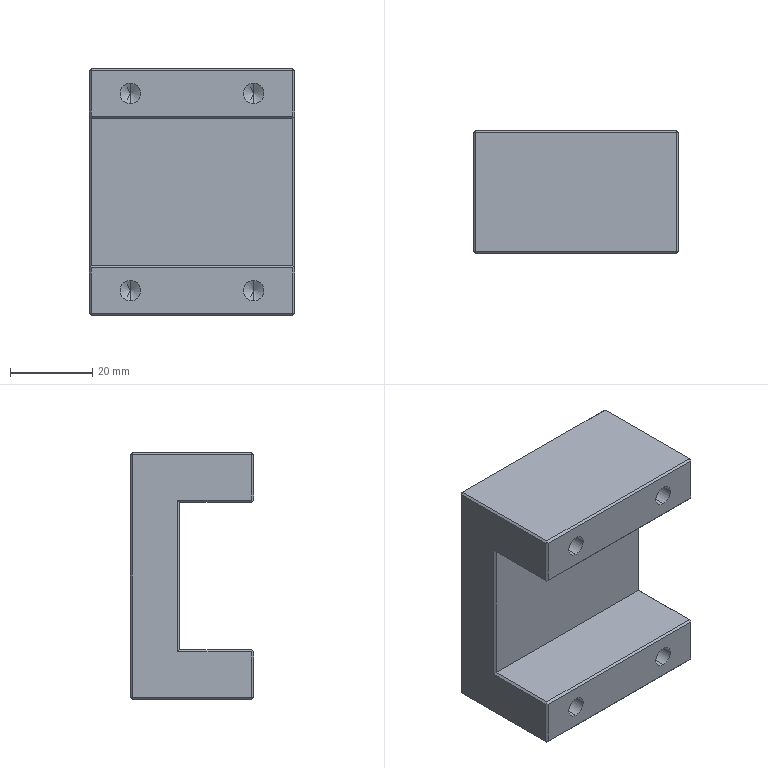Part | SolidWorks | features Chamfer 2, Extrusion 1, HoleWzd 1, ICE 1 | 1 solid | 56 faces | box 50 x 30 x 60 mm | volume 56292 mm3 | plane 40 | cylinder 8 | cone 8 | commonest cylinder face diameters 5 x8
STEP:
#1=CARTESIAN_POINT('',(-15.,15.,-21.5));
#2=VERTEX_POINT('',#1);
#3=CARTESIAN_POINT('',(-15.,15.,-26.5));
#4=VERTEX_POINT('',#3);
#5=CARTESIAN_POINT('',(-15.,15.,-24.));
#6=DIRECTION('',(0.,-1.,0.));
#7=DIRECTION('',(0.,0.,-1.));
#8=AXIS2_PLACEMENT_3D('',#5,#6,#7);
#9=CIRCLE('',#8,2.5);
#10=EDGE_CURVE('',#2,#4,#9,.T.);
#11=ORIENTED_EDGE('',*,*,#10,.F.);
#12=CARTESIAN_POINT('',(-15.,0.,-21.5));
#13=VERTEX_POINT('',#12);
#14=CARTESIAN_POINT('',(-15.,0.,-21.5));
#15=DIRECTION('',(0.,-1.,0.));
#16=VECTOR('',#15,1000.);
#17=LINE('',#14,#16);
#18=EDGE_CURVE('',#2,#13,#17,.T.);
#19=ORIENTED_EDGE('',*,*,#18,.T.);
#20=CARTESIAN_POINT('',(-15.,0.,-26.5));
#21=VERTEX_POINT('',#20);
#22=CARTESIAN_POINT('',(-15.,0.,-24.));
#23=DIRECTION('',(0.,-1.,0.));
#24=DIRECTION('',(0.,0.,-1.));
#25=AXIS2_PLACEMENT_3D('',#22,#23,#24);
#26=CIRCLE('',#25,2.5);
#27=EDGE_CURVE('',#13,#21,#26,.T.);
#28=ORIENTED_EDGE('',*,*,#27,.T.);
#29=CARTESIAN_POINT('',(-15.,0.,-26.5));
#30=DIRECTION('',(0.,-1.,0.));
#31=VECTOR('',#30,1000.);
#32=LINE('',#29,#31);
#33=EDGE_CURVE('',#4,#21,#32,.T.);
#34=ORIENTED_EDGE('',*,*,#33,.F.);
#35=EDGE_LOOP('',(#11,#19,#28,#34));
#36=FACE_OUTER_BOUND('',#35,.T.);
#37=CARTESIAN_POINT('',(-15.,0.,-24.));
#38=DIRECTION('',(0.,-1.,0.));
#39=DIRECTION('',(0.,0.,-1.));
#40=AXIS2_PLACEMENT_3D('',#37,#38,#39);
#41=CYLINDRICAL_SURFACE('',#40,2.5);
#42=ADVANCED_FACE('',(#36),#41,.F.);
#43=CARTESIAN_POINT('',(-15.,16.502,-24.));
#44=VERTEX_POINT('',#43);
#45=CARTESIAN_POINT('',(-15.,15.,-26.5));
#46=DIRECTION('',(0.,-0.515,-0.8572));
#47=VECTOR('',#46,1000.);
#48=LINE('',#45,#47);
#49=EDGE_CURVE('',#44,#4,#48,.T.);
#50=ORIENTED_EDGE('',*,*,#49,.F.);
#51=CARTESIAN_POINT('',(-15.,15.,-21.5));
#52=DIRECTION('',(0.,-0.515,0.8572));
#53=VECTOR('',#52,1000.);
#54=LINE('',#51,#53);
#55=EDGE_CURVE('',#44,#2,#54,.T.);
#56=ORIENTED_EDGE('',*,*,#55,.T.);
#57=ORIENTED_EDGE('',*,*,#10,.T.);
#58=EDGE_LOOP('',(#50,#56,#57));
#59=FACE_OUTER_BOUND('',#58,.T.);
#60=CARTESIAN_POINT('',(-15.,15.,-24.));
#61=DIRECTION('',(0.,-1.,0.));
#62=DIRECTION('',(0.,0.,-1.));
#63=AXIS2_PLACEMENT_3D('',#60,#61,#62);
#64=CONICAL_SURFACE('',#63,2.5,1.03);
#65=ADVANCED_FACE('',(#59),#64,.F.);
#66=CARTESIAN_POINT('',(15.,15.,-21.5));
#67=VERTEX_POINT('',#66);
#68=CARTESIAN_POINT('',(15.,15.,-26.5));
#69=VERTEX_POINT('',#68);
#70=CARTESIAN_POINT('',(15.,15.,-24.));
#71=DIRECTION('',(0.,-1.,0.));
#72=DIRECTION('',(0.,0.,-1.));
#73=AXIS2_PLACEMENT_3D('',#70,#71,#72);
#74=CIRCLE('',#73,2.5);
#75=EDGE_CURVE('',#67,#69,#74,.T.);
#76=ORIENTED_EDGE('',*,*,#75,.F.);
#77=CARTESIAN_POINT('',(15.,0.,-21.5));
#78=VERTEX_POINT('',#77);
#79=CARTESIAN_POINT('',(15.,0.,-21.5));
#80=DIRECTION('',(0.,-1.,0.));
#81=VECTOR('',#80,1000.);
#82=LINE('',#79,#81);
#83=EDGE_CURVE('',#67,#78,#82,.T.);
#84=ORIENTED_EDGE('',*,*,#83,.T.);
#85=CARTESIAN_POINT('',(15.,0.,-26.5));
#86=VERTEX_POINT('',#85);
#87=CARTESIAN_POINT('',(15.,0.,-24.));
#88=DIRECTION('',(0.,-1.,0.));
#89=DIRECTION('',(0.,0.,-1.));
#90=AXIS2_PLACEMENT_3D('',#87,#88,#89);
#91=CIRCLE('',#90,2.5);
#92=EDGE_CURVE('',#78,#86,#91,.T.);
#93=ORIENTED_EDGE('',*,*,#92,.T.);
#94=CARTESIAN_POINT('',(15.,0.,-26.5));
#95=DIRECTION('',(0.,-1.,0.));
#96=VECTOR('',#95,1000.);
#97=LINE('',#94,#96);
#98=EDGE_CURVE('',#69,#86,#97,.T.);
#99=ORIENTED_EDGE('',*,*,#98,.F.);
#100=EDGE_LOOP('',(#76,#84,#93,#99));
#101=FACE_OUTER_BOUND('',#100,.T.);
#102=CARTESIAN_POINT('',(15.,0.,-24.));
#103=DIRECTION('',(0.,-1.,0.));
#104=DIRECTION('',(0.,0.,-1.));
#105=AXIS2_PLACEMENT_3D('',#102,#103,#104);
#106=CYLINDRICAL_SURFACE('',#105,2.5);
#107=ADVANCED_FACE('',(#101),#106,.F.);
#108=CARTESIAN_POINT('',(15.,16.502,-24.));
#109=VERTEX_POINT('',#108);
#110=CARTESIAN_POINT('',(15.,15.,-26.5));
#111=DIRECTION('',(0.,-0.515,-0.8572));
#112=VECTOR('',#111,1000.);
#113=LINE('',#110,#112);
#114=EDGE_CURVE('',#109,#69,#113,.T.);
#115=ORIENTED_EDGE('',*,*,#114,.F.);
#116=CARTESIAN_POINT('',(15.,15.,-21.5));
#117=DIRECTION('',(0.,-0.515,0.8572));
#118=VECTOR('',#117,1000.);
#119=LINE('',#116,#118);
#120=EDGE_CURVE('',#109,#67,#119,.T.);
#121=ORIENTED_EDGE('',*,*,#120,.T.);
#122=ORIENTED_EDGE('',*,*,#75,.T.);
#123=EDGE_LOOP('',(#115,#121,#122));
#124=FACE_OUTER_BOUND('',#123,.T.);
#125=CARTESIAN_POINT('',(15.,15.,-24.));
#126=DIRECTION('',(0.,-1.,0.));
#127=DIRECTION('',(0.,0.,-1.));
#128=AXIS2_PLACEMENT_3D('',#125,#126,#127);
#129=CONICAL_SURFACE('',#128,2.5,1.03);
#130=ADVANCED_FACE('',(#124),#129,.F.);
#131=CARTESIAN_POINT('',(-15.,15.,26.5));
#132=VERTEX_POINT('',#131);
#133=CARTESIAN_POINT('',(-15.,15.,21.5));
#134=VERTEX_POINT('',#133);
#135=CARTESIAN_POINT('',(-15.,15.,24.));
#136=DIRECTION('',(0.,-1.,0.));
#137=DIRECTION('',(0.,0.,-1.));
#138=AXIS2_PLACEMENT_3D('',#135,#136,#137);
#139=CIRCLE('',#138,2.5);
#140=EDGE_CURVE('',#132,#134,#139,.T.);
#141=ORIENTED_EDGE('',*,*,#140,.F.);
#142=CARTESIAN_POINT('',(-15.,0.,26.5));
#143=VERTEX_POINT('',#142);
#144=CARTESIAN_POINT('',(-15.,0.,26.5));
#145=DIRECTION('',(0.,-1.,0.));
#146=VECTOR('',#145,1000.);
#147=LINE('',#144,#146);
#148=EDGE_CURVE('',#132,#143,#147,.T.);
#149=ORIENTED_EDGE('',*,*,#148,.T.);
#150=CARTESIAN_POINT('',(-15.,0.,21.5));
#151=VERTEX_POINT('',#150);
#152=CARTESIAN_POINT('',(-15.,0.,24.));
#153=DIRECTION('',(0.,-1.,0.));
#154=DIRECTION('',(0.,0.,-1.));
#155=AXIS2_PLACEMENT_3D('',#152,#153,#154);
#156=CIRCLE('',#155,2.5);
#157=EDGE_CURVE('',#143,#151,#156,.T.);
#158=ORIENTED_EDGE('',*,*,#157,.T.);
#159=CARTESIAN_POINT('',(-15.,0.,21.5));
#160=DIRECTION('',(0.,-1.,0.));
#161=VECTOR('',#160,1000.);
#162=LINE('',#159,#161);
#163=EDGE_CURVE('',#134,#151,#162,.T.);
#164=ORIENTED_EDGE('',*,*,#163,.F.);
#165=EDGE_LOOP('',(#141,#149,#158,#164));
#166=FACE_OUTER_BOUND('',#165,.T.);
#167=CARTESIAN_POINT('',(-15.,0.,24.));
#168=DIRECTION('',(0.,-1.,0.));
#169=DIRECTION('',(0.,0.,-1.));
#170=AXIS2_PLACEMENT_3D('',#167,#168,#169);
#171=CYLINDRICAL_SURFACE('',#170,2.5);
#172=ADVANCED_FACE('',(#166),#171,.F.);
#173=CARTESIAN_POINT('',(-15.,16.502,24.));
#174=VERTEX_POINT('',#173);
#175=CARTESIAN_POINT('',(-15.,15.,21.5));
#176=DIRECTION('',(0.,-0.515,-0.8572));
#177=VECTOR('',#176,1000.);
#178=LINE('',#175,#177);
#179=EDGE_CURVE('',#174,#134,#178,.T.);
#180=ORIENTED_EDGE('',*,*,#179,.F.);
#181=CARTESIAN_POINT('',(-15.,15.,26.5));
#182=DIRECTION('',(0.,-0.515,0.8572));
#183=VECTOR('',#182,1000.);
#184=LINE('',#181,#183);
#185=EDGE_CURVE('',#174,#132,#184,.T.);
#186=ORIENTED_EDGE('',*,*,#185,.T.);
#187=ORIENTED_EDGE('',*,*,#140,.T.);
#188=EDGE_LOOP('',(#180,#186,#187));
#189=FACE_OUTER_BOUND('',#188,.T.);
#190=CARTESIAN_POINT('',(-15.,15.,24.));
#191=DIRECTION('',(0.,-1.,0.));
#192=DIRECTION('',(0.,0.,-1.));
#193=AXIS2_PLACEMENT_3D('',#190,#191,#192);
#194=CONICAL_SURFACE('',#193,2.5,1.03);
#195=ADVANCED_FACE('',(#189),#194,.F.);
#196=CARTESIAN_POINT('',(15.,15.,26.5));
#197=VERTEX_POINT('',#196);
#198=CARTESIAN_POINT('',(15.,15.,21.5));
#199=VERTEX_POINT('',#198);
#200=CARTESIAN_POINT('',(15.,15.,24.));
#201=DIRECTION('',(0.,-1.,0.));
#202=DIRECTION('',(0.,0.,-1.));
#203=AXIS2_PLACEMENT_3D('',#200,#201,#202);
#204=CIRCLE('',#203,2.5);
#205=EDGE_CURVE('',#197,#199,#204,.T.);
#206=ORIENTED_EDGE('',*,*,#205,.F.);
#207=CARTESIAN_POINT('',(15.,0.,26.5));
#208=VERTEX_POINT('',#207);
#209=CARTESIAN_POINT('',(15.,0.,26.5));
#210=DIRECTION('',(0.,-1.,0.));
#211=VECTOR('',#210,1000.);
#212=LINE('',#209,#211);
#213=EDGE_CURVE('',#197,#208,#212,.T.);
#214=ORIENTED_EDGE('',*,*,#213,.T.);
#215=CARTESIAN_POINT('',(15.,0.,21.5));
#216=VERTEX_POINT('',#215);
#217=CARTESIAN_POINT('',(15.,0.,24.));
#218=DIRECTION('',(0.,-1.,0.));
#219=DIRECTION('',(0.,0.,-1.));
#220=AXIS2_PLACEMENT_3D('',#217,#218,#219);
#221=CIRCLE('',#220,2.5);
#222=EDGE_CURVE('',#208,#216,#221,.T.);
#223=ORIENTED_EDGE('',*,*,#222,.T.);
#224=CARTESIAN_POINT('',(15.,0.,21.5));
#225=DIRECTION('',(0.,-1.,0.));
#226=VECTOR('',#225,1000.);
#227=LINE('',#224,#226);
#228=EDGE_CURVE('',#199,#216,#227,.T.);
#229=ORIENTED_EDGE('',*,*,#228,.F.);
#230=EDGE_LOOP('',(#206,#214,#223,#229));
#231=FACE_OUTER_BOUND('',#230,.T.);
#232=CARTESIAN_POINT('',(15.,0.,24.));
#233=DIRECTION('',(0.,-1.,0.));
#234=DIRECTION('',(0.,0.,-1.));
#235=AXIS2_PLACEMENT_3D('',#232,#233,#234);
#236=CYLINDRICAL_SURFACE('',#235,2.5);
#237=ADVANCED_FACE('',(#231),#236,.F.);
#238=CARTESIAN_POINT('',(15.,16.502,24.));
#239=VERTEX_POINT('',#238);
#240=CARTESIAN_POINT('',(15.,15.,21.5));
#241=DIRECTION('',(0.,-0.515,-0.8572));
#242=VECTOR('',#241,1000.);
#243=LINE('',#240,#242);
#244=EDGE_CURVE('',#239,#199,#243,.T.);
#245=ORIENTED_EDGE('',*,*,#244,.F.);
#246=CARTESIAN_POINT('',(15.,15.,26.5));
#247=DIRECTION('',(0.,-0.515,0.8572));
#248=VECTOR('',#247,1000.);
#249=LINE('',#246,#248);
#250=EDGE_CURVE('',#239,#197,#249,.T.);
#251=ORIENTED_EDGE('',*,*,#250,.T.);
#252=ORIENTED_EDGE('',*,*,#205,.T.);
#253=EDGE_LOOP('',(#245,#251,#252));
#254=FACE_OUTER_BOUND('',#253,.T.);
#255=CARTESIAN_POINT('',(15.,15.,24.));
#256=DIRECTION('',(0.,-1.,0.));
#257=DIRECTION('',(0.,0.,-1.));
#258=AXIS2_PLACEMENT_3D('',#255,#256,#257);
#259=CONICAL_SURFACE('',#258,2.5,1.03);
#260=ADVANCED_FACE('',(#254),#259,.F.);
#261=CARTESIAN_POINT('',(-15.,0.,-24.));
#262=DIRECTION('',(0.,-1.,0.));
#263=DIRECTION('',(0.,0.,-1.));
#264=AXIS2_PLACEMENT_3D('',#261,#262,#263);
#265=CIRCLE('',#264,2.5);
#266=EDGE_CURVE('',#21,#13,#265,.T.);
#267=ORIENTED_EDGE('',*,*,#266,.F.);
#268=ORIENTED_EDGE('',*,*,#27,.F.);
#269=EDGE_LOOP('',(#267,#268));
#270=FACE_BOUND('',#269,.T.);
#271=CARTESIAN_POINT('',(15.,0.,-24.));
#272=DIRECTION('',(0.,-1.,0.));
#273=DIRECTION('',(0.,0.,-1.));
#274=AXIS2_PLACEMENT_3D('',#271,#272,#273);
#275=CIRCLE('',#274,2.5);
#276=EDGE_CURVE('',#86,#78,#275,.T.);
#277=ORIENTED_EDGE('',*,*,#276,.F.);
#278=ORIENTED_EDGE('',*,*,#92,.F.);
#279=EDGE_LOOP('',(#277,#278));
#280=FACE_BOUND('',#279,.T.);
#281=CARTESIAN_POINT('',(24.5,0.,-29.5));
#282=VERTEX_POINT('',#281);
#283=CARTESIAN_POINT('',(24.5,0.,-18.5));
#284=VERTEX_POINT('',#283);
#285=CARTESIAN_POINT('',(24.5,0.,30.));
#286=DIRECTION('',(0.,0.,1.));
#287=VECTOR('',#286,1000.);
#288=LINE('',#285,#287);
#289=EDGE_CURVE('',#282,#284,#288,.T.);
#290=ORIENTED_EDGE('',*,*,#289,.T.);
#291=CARTESIAN_POINT('',(-24.5,0.,-18.5));
#292=VERTEX_POINT('',#291);
#293=CARTESIAN_POINT('',(-24.5,0.,-18.5));
#294=DIRECTION('',(-1.,0.,0.));
#295=VECTOR('',#294,1000.);
#296=LINE('',#293,#295);
#297=EDGE_CURVE('',#284,#292,#296,.T.);
#298=ORIENTED_EDGE('',*,*,#297,.T.);
#299=CARTESIAN_POINT('',(-24.5,0.,-29.5));
#300=VERTEX_POINT('',#299);
#301=CARTESIAN_POINT('',(-24.5,0.,-30.));
#302=DIRECTION('',(0.,0.,-1.));
#303=VECTOR('',#302,1000.);
#304=LINE('',#301,#303);
#305=EDGE_CURVE('',#292,#300,#304,.T.);
#306=ORIENTED_EDGE('',*,*,#305,.T.);
#307=CARTESIAN_POINT('',(25.,0.,-29.5));
#308=DIRECTION('',(1.,0.,0.));
#309=VECTOR('',#308,1000.);
#310=LINE('',#307,#309);
#311=EDGE_CURVE('',#300,#282,#310,.T.);
#312=ORIENTED_EDGE('',*,*,#311,.T.);
#313=EDGE_LOOP('',(#290,#298,#306,#312));
#314=FACE_OUTER_BOUND('',#313,.T.);
#315=CARTESIAN_POINT('',(0.,0.,0.));
#316=DIRECTION('',(0.,-1.,0.));
#317=DIRECTION('',(0.,0.,-1.));
#318=AXIS2_PLACEMENT_3D('',#315,#316,#317);
#319=PLANE('',#318);
#320=ADVANCED_FACE('',(#270,#280,#314),#319,.T.);
#321=ORIENTED_EDGE('',*,*,#305,.F.);
#322=CARTESIAN_POINT('',(-24.75,0.25,-18.25));
#323=VERTEX_POINT('',#322);
#324=CARTESIAN_POINT('',(-41.,16.5,-2.));
#325=DIRECTION('',(-0.5774,0.5774,0.5774));
#326=VECTOR('',#325,1000.);
#327=LINE('',#324,#326);
#328=EDGE_CURVE('',#292,#323,#327,.T.);
#329=ORIENTED_EDGE('',*,*,#328,.T.);
#330=CARTESIAN_POINT('',(-25.,0.5,-18.5));
#331=VERTEX_POINT('',#330);
#332=CARTESIAN_POINT('',(-8.833,-15.667,-2.333));
#333=DIRECTION('',(-0.5774,0.5774,-0.5774));
#334=VECTOR('',#333,1000.);
#335=LINE('',#332,#334);
#336=EDGE_CURVE('',#323,#331,#335,.T.);
#337=ORIENTED_EDGE('',*,*,#336,.T.);
#338=CARTESIAN_POINT('',(-25.,0.5,-29.5));
#339=VERTEX_POINT('',#338);
#340=CARTESIAN_POINT('',(-25.,0.5,30.));
#341=DIRECTION('',(0.,0.,1.));
#342=VECTOR('',#341,1000.);
#343=LINE('',#340,#342);
#344=EDGE_CURVE('',#339,#331,#343,.T.);
#345=ORIENTED_EDGE('',*,*,#344,.F.);
#346=CARTESIAN_POINT('',(-25.,0.5,-29.5));
#347=DIRECTION('',(-0.7071,0.7071,0.));
#348=VECTOR('',#347,1000.);
#349=LINE('',#346,#348);
#350=EDGE_CURVE('',#300,#339,#349,.T.);
#351=ORIENTED_EDGE('',*,*,#350,.F.);
#352=EDGE_LOOP('',(#321,#329,#337,#345,#351));
#353=FACE_OUTER_BOUND('',#352,.T.);
#354=CARTESIAN_POINT('',(-25.,0.5,30.));
#355=DIRECTION('',(-0.7071,-0.7071,0.));
#356=DIRECTION('',(0.,0.,-1.));
#357=AXIS2_PLACEMENT_3D('',#354,#355,#356);
#358=PLANE('',#357);
#359=ADVANCED_FACE('',(#353),#358,.T.);
#360=CARTESIAN_POINT('',(25.,0.5,-18.5));
#361=VERTEX_POINT('',#360);
#362=CARTESIAN_POINT('',(24.75,0.25,-18.25));
#363=VERTEX_POINT('',#362);
#364=CARTESIAN_POINT('',(8.833,-15.667,-2.333));
#365=DIRECTION('',(-0.5774,-0.5774,0.5774));
#366=VECTOR('',#365,1000.);
#367=LINE('',#364,#366);
#368=EDGE_CURVE('',#361,#363,#367,.T.);
#369=ORIENTED_EDGE('',*,*,#368,.T.);
#370=CARTESIAN_POINT('',(41.,16.5,-2.));
#371=DIRECTION('',(-0.5774,-0.5774,-0.5774));
#372=VECTOR('',#371,1000.);
#373=LINE('',#370,#372);
#374=EDGE_CURVE('',#363,#284,#373,.T.);
#375=ORIENTED_EDGE('',*,*,#374,.T.);
#376=ORIENTED_EDGE('',*,*,#289,.F.);
#377=CARTESIAN_POINT('',(25.,0.5,-29.5));
#378=VERTEX_POINT('',#377);
#379=CARTESIAN_POINT('',(24.75,0.25,-29.5));
#380=DIRECTION('',(-0.7071,-0.7071,0.));
#381=VECTOR('',#380,1000.);
#382=LINE('',#379,#381);
#383=EDGE_CURVE('',#378,#282,#382,.T.);
#384=ORIENTED_EDGE('',*,*,#383,.F.);
#385=CARTESIAN_POINT('',(25.,0.5,-30.));
#386=DIRECTION('',(0.,0.,-1.));
#387=VECTOR('',#386,1000.);
#388=LINE('',#385,#387);
#389=EDGE_CURVE('',#361,#378,#388,.T.);
#390=ORIENTED_EDGE('',*,*,#389,.F.);
#391=EDGE_LOOP('',(#369,#375,#376,#384,#390));
#392=FACE_OUTER_BOUND('',#391,.T.);
#393=CARTESIAN_POINT('',(25.,0.5,30.));
#394=DIRECTION('',(0.7071,-0.7071,0.));
#395=DIRECTION('',(0.,0.,1.));
#396=AXIS2_PLACEMENT_3D('',#393,#394,#395);
#397=PLANE('',#396);
#398=ADVANCED_FACE('',(#392),#397,.T.);
#399=CARTESIAN_POINT('',(25.,18.5,18.5));
#400=VERTEX_POINT('',#399);
#401=CARTESIAN_POINT('',(25.,18.5,-18.5));
#402=VERTEX_POINT('',#401);
#403=CARTESIAN_POINT('',(25.,18.5,30.));
#404=DIRECTION('',(0.,0.,-1.));
#405=VECTOR('',#404,1000.);
#406=LINE('',#403,#405);
#407=EDGE_CURVE('',#400,#402,#406,.T.);
#408=ORIENTED_EDGE('',*,*,#407,.T.);
#409=CARTESIAN_POINT('',(25.,30.,-18.5));
#410=DIRECTION('',(0.,-1.,0.));
#411=VECTOR('',#410,1000.);
#412=LINE('',#409,#411);
#413=EDGE_CURVE('',#402,#361,#412,.T.);
#414=ORIENTED_EDGE('',*,*,#413,.T.);
#415=ORIENTED_EDGE('',*,*,#389,.T.);
#416=CARTESIAN_POINT('',(25.,29.5,-29.5));
#417=VERTEX_POINT('',#416);
#418=CARTESIAN_POINT('',(25.,30.,-29.5));
#419=DIRECTION('',(0.,1.,0.));
#420=VECTOR('',#419,1000.);
#421=LINE('',#418,#420);
#422=EDGE_CURVE('',#378,#417,#421,.T.);
#423=ORIENTED_EDGE('',*,*,#422,.T.);
#424=CARTESIAN_POINT('',(25.,29.5,29.5));
#425=VERTEX_POINT('',#424);
#426=CARTESIAN_POINT('',(25.,29.5,30.));
#427=DIRECTION('',(0.,0.,1.));
#428=VECTOR('',#427,1000.);
#429=LINE('',#426,#428);
#430=EDGE_CURVE('',#417,#425,#429,.T.);
#431=ORIENTED_EDGE('',*,*,#430,.T.);
#432=CARTESIAN_POINT('',(25.,0.5,29.5));
#433=VERTEX_POINT('',#432);
#434=CARTESIAN_POINT('',(25.,30.,29.5));
#435=DIRECTION('',(0.,-1.,0.));
#436=VECTOR('',#435,1000.);
#437=LINE('',#434,#436);
#438=EDGE_CURVE('',#425,#433,#437,.T.);
#439=ORIENTED_EDGE('',*,*,#438,.T.);
#440=CARTESIAN_POINT('',(25.,0.5,18.5));
#441=VERTEX_POINT('',#440);
#442=CARTESIAN_POINT('',(25.,0.5,-30.));
#443=DIRECTION('',(0.,0.,-1.));
#444=VECTOR('',#443,1000.);
#445=LINE('',#442,#444);
#446=EDGE_CURVE('',#433,#441,#445,.T.);
#447=ORIENTED_EDGE('',*,*,#446,.T.);
#448=CARTESIAN_POINT('',(25.,30.,18.5));
#449=DIRECTION('',(0.,1.,0.));
#450=VECTOR('',#449,1000.);
#451=LINE('',#448,#450);
#452=EDGE_CURVE('',#441,#400,#451,.T.);
#453=ORIENTED_EDGE('',*,*,#452,.T.);
#454=EDGE_LOOP('',(#408,#414,#415,#423,#431,#439,#447,#453));
#455=FACE_OUTER_BOUND('',#454,.T.);
#456=CARTESIAN_POINT('',(25.,30.,30.));
#457=DIRECTION('',(-1.,0.,0.));
#458=DIRECTION('',(0.,0.,1.));
#459=AXIS2_PLACEMENT_3D('',#456,#457,#458);
#460=PLANE('',#459);
#461=ADVANCED_FACE('',(#455),#460,.F.);
#462=CARTESIAN_POINT('',(-24.5,0.5,-30.));
#463=VERTEX_POINT('',#462);
#464=CARTESIAN_POINT('',(-24.5,29.5,-30.));
#465=VERTEX_POINT('',#464);
#466=CARTESIAN_POINT('',(-24.5,30.,-30.));
#467=DIRECTION('',(0.,1.,0.));
#468=VECTOR('',#467,1000.);
#469=LINE('',#466,#468);
#470=EDGE_CURVE('',#463,#465,#469,.T.);
#471=ORIENTED_EDGE('',*,*,#470,.T.);
#472=CARTESIAN_POINT('',(24.5,29.5,-30.));
#473=VERTEX_POINT('',#472);
#474=CARTESIAN_POINT('',(-25.,29.5,-30.));
#475=DIRECTION('',(1.,0.,0.));
#476=VECTOR('',#475,1000.);
#477=LINE('',#474,#476);
#478=EDGE_CURVE('',#465,#473,#477,.T.);
#479=ORIENTED_EDGE('',*,*,#478,.T.);
#480=CARTESIAN_POINT('',(24.5,0.5,-30.));
#481=VERTEX_POINT('',#480);
#482=CARTESIAN_POINT('',(24.5,30.,-30.));
#483=DIRECTION('',(0.,-1.,0.));
#484=VECTOR('',#483,1000.);
#485=LINE('',#482,#484);
#486=EDGE_CURVE('',#473,#481,#485,.T.);
#487=ORIENTED_EDGE('',*,*,#486,.T.);
#488=CARTESIAN_POINT('',(-25.,0.5,-30.));
#489=DIRECTION('',(-1.,0.,0.));
#490=VECTOR('',#489,1000.);
#491=LINE('',#488,#490);
#492=EDGE_CURVE('',#481,#463,#491,.T.);
#493=ORIENTED_EDGE('',*,*,#492,.T.);
#494=EDGE_LOOP('',(#471,#479,#487,#493));
#495=FACE_OUTER_BOUND('',#494,.T.);
#496=CARTESIAN_POINT('',(-25.,30.,-30.));
#497=DIRECTION('',(0.,0.,1.));
#498=DIRECTION('',(1.,0.,0.));
#499=AXIS2_PLACEMENT_3D('',#496,#497,#498);
#500=PLANE('',#499);
#501=ADVANCED_FACE('',(#495),#500,.F.);
#502=CARTESIAN_POINT('',(-25.,18.5,-18.5));
#503=VERTEX_POINT('',#502);
#504=CARTESIAN_POINT('',(-25.,18.5,18.5));
#505=VERTEX_POINT('',#504);
#506=CARTESIAN_POINT('',(-25.,18.5,30.));
#507=DIRECTION('',(0.,0.,1.));
#508=VECTOR('',#507,1000.);
#509=LINE('',#506,#508);
#510=EDGE_CURVE('',#503,#505,#509,.T.);
#511=ORIENTED_EDGE('',*,*,#510,.T.);
#512=CARTESIAN_POINT('',(-25.,0.5,18.5));
#513=VERTEX_POINT('',#512);
#514=CARTESIAN_POINT('',(-25.,30.,18.5));
#515=DIRECTION('',(0.,-1.,0.));
#516=VECTOR('',#515,1000.);
#517=LINE('',#514,#516);
#518=EDGE_CURVE('',#505,#513,#517,.T.);
#519=ORIENTED_EDGE('',*,*,#518,.T.);
#520=CARTESIAN_POINT('',(-25.,0.5,29.5));
#521=VERTEX_POINT('',#520);
#522=CARTESIAN_POINT('',(-25.,0.5,30.));
#523=DIRECTION('',(0.,0.,1.));
#524=VECTOR('',#523,1000.);
#525=LINE('',#522,#524);
#526=EDGE_CURVE('',#513,#521,#525,.T.);
#527=ORIENTED_EDGE('',*,*,#526,.T.);
#528=CARTESIAN_POINT('',(-25.,29.5,29.5));
#529=VERTEX_POINT('',#528);
#530=CARTESIAN_POINT('',(-25.,30.,29.5));
#531=DIRECTION('',(0.,1.,0.));
#532=VECTOR('',#531,1000.);
#533=LINE('',#530,#532);
#534=EDGE_CURVE('',#521,#529,#533,.T.);
#535=ORIENTED_EDGE('',*,*,#534,.T.);
#536=CARTESIAN_POINT('',(-25.,29.5,-29.5));
#537=VERTEX_POINT('',#536);
#538=CARTESIAN_POINT('',(-25.,29.5,30.));
#539=DIRECTION('',(0.,0.,-1.));
#540=VECTOR('',#539,1000.);
#541=LINE('',#538,#540);
#542=EDGE_CURVE('',#529,#537,#541,.T.);
#543=ORIENTED_EDGE('',*,*,#542,.T.);
#544=CARTESIAN_POINT('',(-25.,30.,-29.5));
#545=DIRECTION('',(0.,-1.,0.));
#546=VECTOR('',#545,1000.);
#547=LINE('',#544,#546);
#548=EDGE_CURVE('',#537,#339,#547,.T.);
#549=ORIENTED_EDGE('',*,*,#548,.T.);
#550=ORIENTED_EDGE('',*,*,#344,.T.);
#551=CARTESIAN_POINT('',(-25.,30.,-18.5));
#552=DIRECTION('',(0.,1.,0.));
#553=VECTOR('',#552,1000.);
#554=LINE('',#551,#553);
#555=EDGE_CURVE('',#331,#503,#554,.T.);
#556=ORIENTED_EDGE('',*,*,#555,.T.);
#557=EDGE_LOOP('',(#511,#519,#527,#535,#543,#549,#550,#556));
#558=FACE_OUTER_BOUND('',#557,.T.);
#559=CARTESIAN_POINT('',(-25.,30.,30.));
#560=DIRECTION('',(1.,0.,0.));
#561=DIRECTION('',(0.,0.,-1.));
#562=AXIS2_PLACEMENT_3D('',#559,#560,#561);
#563=PLANE('',#562);
#564=ADVANCED_FACE('',(#558),#563,.F.);
#565=CARTESIAN_POINT('',(24.5,29.5,30.));
#566=VERTEX_POINT('',#565);
#567=CARTESIAN_POINT('',(-24.5,29.5,30.));
#568=VERTEX_POINT('',#567);
#569=CARTESIAN_POINT('',(-25.,29.5,30.));
#570=DIRECTION('',(-1.,0.,0.));
#571=VECTOR('',#570,1000.);
#572=LINE('',#569,#571);
#573=EDGE_CURVE('',#566,#568,#572,.T.);
#574=ORIENTED_EDGE('',*,*,#573,.T.);
#575=CARTESIAN_POINT('',(-24.5,0.5,30.));
#576=VERTEX_POINT('',#575);
#577=CARTESIAN_POINT('',(-24.5,30.,30.));
#578=DIRECTION('',(0.,-1.,0.));
#579=VECTOR('',#578,1000.);
#580=LINE('',#577,#579);
#581=EDGE_CURVE('',#568,#576,#580,.T.);
#582=ORIENTED_EDGE('',*,*,#581,.T.);
#583=CARTESIAN_POINT('',(24.5,0.5,30.));
#584=VERTEX_POINT('',#583);
#585=CARTESIAN_POINT('',(25.,0.5,30.));
#586=DIRECTION('',(1.,0.,0.));
#587=VECTOR('',#586,1000.);
#588=LINE('',#585,#587);
#589=EDGE_CURVE('',#576,#584,#588,.T.);
#590=ORIENTED_EDGE('',*,*,#589,.T.);
#591=CARTESIAN_POINT('',(24.5,30.,30.));
#592=DIRECTION('',(0.,1.,0.));
#593=VECTOR('',#592,1000.);
#594=LINE('',#591,#593);
#595=EDGE_CURVE('',#584,#566,#594,.T.);
#596=ORIENTED_EDGE('',*,*,#595,.T.);
#597=EDGE_LOOP('',(#574,#582,#590,#596));
#598=FACE_OUTER_BOUND('',#597,.T.);
#599=CARTESIAN_POINT('',(-25.,30.,30.));
#600=DIRECTION('',(0.,0.,-1.));
#601=DIRECTION('',(-1.,0.,0.));
#602=AXIS2_PLACEMENT_3D('',#599,#600,#601);
#603=PLANE('',#602);
#604=ADVANCED_FACE('',(#598),#603,.F.);
#605=CARTESIAN_POINT('',(-24.5,30.,-29.5));
#606=VERTEX_POINT('',#605);
#607=CARTESIAN_POINT('',(-24.5,30.,29.5));
#608=VERTEX_POINT('',#607);
#609=CARTESIAN_POINT('',(-24.5,30.,0.));
#610=DIRECTION('',(0.,0.,1.));
#611=VECTOR('',#610,1000.);
#612=LINE('',#609,#611);
#613=EDGE_CURVE('',#606,#608,#612,.T.);
#614=ORIENTED_EDGE('',*,*,#613,.T.);
#615=CARTESIAN_POINT('',(24.5,30.,29.5));
#616=VERTEX_POINT('',#615);
#617=CARTESIAN_POINT('',(0.,30.,29.5));
#618=DIRECTION('',(1.,0.,0.));
#619=VECTOR('',#618,1000.);
#620=LINE('',#617,#619);
#621=EDGE_CURVE('',#608,#616,#620,.T.);
#622=ORIENTED_EDGE('',*,*,#621,.T.);
#623=CARTESIAN_POINT('',(24.5,30.,-29.5));
#624=VERTEX_POINT('',#623);
#625=CARTESIAN_POINT('',(24.5,30.,0.));
#626=DIRECTION('',(0.,0.,-1.));
#627=VECTOR('',#626,1000.);
#628=LINE('',#625,#627);
#629=EDGE_CURVE('',#616,#624,#628,.T.);
#630=ORIENTED_EDGE('',*,*,#629,.T.);
#631=CARTESIAN_POINT('',(0.,30.,-29.5));
#632=DIRECTION('',(-1.,0.,0.));
#633=VECTOR('',#632,1000.);
#634=LINE('',#631,#633);
#635=EDGE_CURVE('',#624,#606,#634,.T.);
#636=ORIENTED_EDGE('',*,*,#635,.T.);
#637=EDGE_LOOP('',(#614,#622,#630,#636));
#638=FACE_OUTER_BOUND('',#637,.T.);
#639=CARTESIAN_POINT('',(0.,30.,0.));
#640=DIRECTION('',(0.,-1.,0.));
#641=DIRECTION('',(0.,0.,-1.));
#642=AXIS2_PLACEMENT_3D('',#639,#640,#641);
#643=PLANE('',#642);
#644=ADVANCED_FACE('',(#638),#643,.F.);
#645=CARTESIAN_POINT('',(-15.,0.,24.));
#646=DIRECTION('',(0.,-1.,0.));
#647=DIRECTION('',(0.,0.,-1.));
#648=AXIS2_PLACEMENT_3D('',#645,#646,#647);
#649=CIRCLE('',#648,2.5);
#650=EDGE_CURVE('',#151,#143,#649,.T.);
#651=ORIENTED_EDGE('',*,*,#650,.F.);
#652=ORIENTED_EDGE('',*,*,#157,.F.);
#653=EDGE_LOOP('',(#651,#652));
#654=FACE_BOUND('',#653,.T.);
#655=CARTESIAN_POINT('',(15.,0.,24.));
#656=DIRECTION('',(0.,-1.,0.));
#657=DIRECTION('',(0.,0.,-1.));
#658=AXIS2_PLACEMENT_3D('',#655,#656,#657);
#659=CIRCLE('',#658,2.5);
#660=EDGE_CURVE('',#216,#208,#659,.T.);
#661=ORIENTED_EDGE('',*,*,#660,.F.);
#662=ORIENTED_EDGE('',*,*,#222,.F.);
#663=EDGE_LOOP('',(#661,#662));
#664=FACE_BOUND('',#663,.T.);
#665=CARTESIAN_POINT('',(-24.5,0.,29.5));
#666=VERTEX_POINT('',#665);
#667=CARTESIAN_POINT('',(-24.5,0.,18.5));
#668=VERTEX_POINT('',#667);
#669=CARTESIAN_POINT('',(-24.5,0.,-30.));
#670=DIRECTION('',(0.,0.,-1.));
#671=VECTOR('',#670,1000.);
#672=LINE('',#669,#671);
#673=EDGE_CURVE('',#666,#668,#672,.T.);
#674=ORIENTED_EDGE('',*,*,#673,.T.);
#675=CARTESIAN_POINT('',(24.5,0.,18.5));
#676=VERTEX_POINT('',#675);
#677=CARTESIAN_POINT('',(24.5,0.,18.5));
#678=DIRECTION('',(1.,0.,0.));
#679=VECTOR('',#678,1000.);
#680=LINE('',#677,#679);
#681=EDGE_CURVE('',#668,#676,#680,.T.);
#682=ORIENTED_EDGE('',*,*,#681,.T.);
#683=CARTESIAN_POINT('',(24.5,0.,29.5));
#684=VERTEX_POINT('',#683);
#685=CARTESIAN_POINT('',(24.5,0.,30.));
#686=DIRECTION('',(0.,0.,1.));
#687=VECTOR('',#686,1000.);
#688=LINE('',#685,#687);
#689=EDGE_CURVE('',#676,#684,#688,.T.);
#690=ORIENTED_EDGE('',*,*,#689,.T.);
#691=CARTESIAN_POINT('',(-25.,0.,29.5));
#692=DIRECTION('',(-1.,0.,0.));
#693=VECTOR('',#692,1000.);
#694=LINE('',#691,#693);
#695=EDGE_CURVE('',#684,#666,#694,.T.);
#696=ORIENTED_EDGE('',*,*,#695,.T.);
#697=EDGE_LOOP('',(#674,#682,#690,#696));
#698=FACE_OUTER_BOUND('',#697,.T.);
#699=CARTESIAN_POINT('',(0.,0.,0.));
#700=DIRECTION('',(0.,-1.,0.));
#701=DIRECTION('',(0.,0.,-1.));
#702=AXIS2_PLACEMENT_3D('',#699,#700,#701);
#703=PLANE('',#702);
#704=ADVANCED_FACE('',(#654,#664,#698),#703,.T.);
#705=CARTESIAN_POINT('',(-25.,29.5,29.5));
#706=DIRECTION('',(0.7071,0.,0.7071));
#707=VECTOR('',#706,1000.);
#708=LINE('',#705,#707);
#709=EDGE_CURVE('',#529,#568,#708,.T.);
#710=ORIENTED_EDGE('',*,*,#709,.F.);
#711=ORIENTED_EDGE('',*,*,#534,.F.);
#712=CARTESIAN_POINT('',(-24.5,0.5,30.));
#713=DIRECTION('',(-0.7071,0.,-0.7071));
#714=VECTOR('',#713,1000.);
#715=LINE('',#712,#714);
#716=EDGE_CURVE('',#576,#521,#715,.T.);
#717=ORIENTED_EDGE('',*,*,#716,.F.);
#718=ORIENTED_EDGE('',*,*,#581,.F.);
#719=EDGE_LOOP('',(#710,#711,#717,#718));
#720=FACE_OUTER_BOUND('',#719,.T.);
#721=CARTESIAN_POINT('',(-24.5,30.,30.));
#722=DIRECTION('',(0.7071,0.,-0.7071));
#723=DIRECTION('',(0.,-1.,0.));
#724=AXIS2_PLACEMENT_3D('',#721,#722,#723);
#725=PLANE('',#724);
#726=ADVANCED_FACE('',(#720),#725,.F.);
#727=CARTESIAN_POINT('',(-25.,29.5,29.5));
#728=DIRECTION('',(0.7071,0.7071,0.));
#729=VECTOR('',#728,1000.);
#730=LINE('',#727,#729);
#731=EDGE_CURVE('',#529,#608,#730,.T.);
#732=ORIENTED_EDGE('',*,*,#731,.F.);
#733=ORIENTED_EDGE('',*,*,#709,.T.);
#734=CARTESIAN_POINT('',(-24.5,29.75,29.75));
#735=DIRECTION('',(0.,-0.7071,0.7071));
#736=VECTOR('',#735,1000.);
#737=LINE('',#734,#736);
#738=EDGE_CURVE('',#608,#568,#737,.T.);
#739=ORIENTED_EDGE('',*,*,#738,.F.);
#740=EDGE_LOOP('',(#732,#733,#739));
#741=FACE_OUTER_BOUND('',#740,.T.);
#742=CARTESIAN_POINT('',(-25.,29.5,29.5));
#743=DIRECTION('',(-0.5774,0.5774,0.5774));
#744=DIRECTION('',(0.7071,0.,0.7071));
#745=AXIS2_PLACEMENT_3D('',#742,#743,#744);
#746=PLANE('',#745);
#747=ADVANCED_FACE('',(#741),#746,.T.);
#748=CARTESIAN_POINT('',(-24.5,0.5,30.));
#749=DIRECTION('',(0.,-0.7071,-0.7071));
#750=VECTOR('',#749,1000.);
#751=LINE('',#748,#750);
#752=EDGE_CURVE('',#576,#666,#751,.T.);
#753=ORIENTED_EDGE('',*,*,#752,.F.);
#754=ORIENTED_EDGE('',*,*,#716,.T.);
#755=CARTESIAN_POINT('',(-24.75,0.25,29.5));
#756=DIRECTION('',(-0.7071,0.7071,0.));
#757=VECTOR('',#756,1000.);
#758=LINE('',#755,#757);
#759=EDGE_CURVE('',#666,#521,#758,.T.);
#760=ORIENTED_EDGE('',*,*,#759,.F.);
#761=EDGE_LOOP('',(#753,#754,#760));
#762=FACE_OUTER_BOUND('',#761,.T.);
#763=CARTESIAN_POINT('',(-24.5,0.5,30.));
#764=DIRECTION('',(-0.5774,-0.5774,0.5774));
#765=DIRECTION('',(0.7071,-0.7071,0.));
#766=AXIS2_PLACEMENT_3D('',#763,#764,#765);
#767=PLANE('',#766);
#768=ADVANCED_FACE('',(#762),#767,.T.);
#769=ORIENTED_EDGE('',*,*,#738,.T.);
#770=ORIENTED_EDGE('',*,*,#573,.F.);
#771=CARTESIAN_POINT('',(24.5,30.,29.5));
#772=DIRECTION('',(0.,-0.7071,0.7071));
#773=VECTOR('',#772,1000.);
#774=LINE('',#771,#773);
#775=EDGE_CURVE('',#616,#566,#774,.T.);
#776=ORIENTED_EDGE('',*,*,#775,.F.);
#777=ORIENTED_EDGE('',*,*,#621,.F.);
#778=EDGE_LOOP('',(#769,#770,#776,#777));
#779=FACE_OUTER_BOUND('',#778,.T.);
#780=CARTESIAN_POINT('',(0.,30.,29.5));
#781=DIRECTION('',(0.,-0.7071,-0.7071));
#782=DIRECTION('',(1.,0.,0.));
#783=AXIS2_PLACEMENT_3D('',#780,#781,#782);
#784=PLANE('',#783);
#785=ADVANCED_FACE('',(#779),#784,.F.);
#786=ORIENTED_EDGE('',*,*,#731,.T.);
#787=ORIENTED_EDGE('',*,*,#613,.F.);
#788=CARTESIAN_POINT('',(-24.75,29.75,-29.5));
#789=DIRECTION('',(0.7071,0.7071,0.));
#790=VECTOR('',#789,1000.);
#791=LINE('',#788,#790);
#792=EDGE_CURVE('',#537,#606,#791,.T.);
#793=ORIENTED_EDGE('',*,*,#792,.F.);
#794=ORIENTED_EDGE('',*,*,#542,.F.);
#795=EDGE_LOOP('',(#786,#787,#793,#794));
#796=FACE_OUTER_BOUND('',#795,.T.);
#797=CARTESIAN_POINT('',(-24.5,30.,0.));
#798=DIRECTION('',(0.7071,-0.7071,0.));
#799=DIRECTION('',(0.,0.,1.));
#800=AXIS2_PLACEMENT_3D('',#797,#798,#799);
#801=PLANE('',#800);
#802=ADVANCED_FACE('',(#796),#801,.F.);
#803=CARTESIAN_POINT('',(-25.,0.5,-29.5));
#804=DIRECTION('',(0.7071,0.,-0.7071));
#805=VECTOR('',#804,1000.);
#806=LINE('',#803,#805);
#807=EDGE_CURVE('',#339,#463,#806,.T.);
#808=ORIENTED_EDGE('',*,*,#807,.F.);
#809=ORIENTED_EDGE('',*,*,#548,.F.);
#810=CARTESIAN_POINT('',(-24.5,29.5,-30.));
#811=DIRECTION('',(-0.7071,0.,0.7071));
#812=VECTOR('',#811,1000.);
#813=LINE('',#810,#812);
#814=EDGE_CURVE('',#465,#537,#813,.T.);
#815=ORIENTED_EDGE('',*,*,#814,.F.);
#816=ORIENTED_EDGE('',*,*,#470,.F.);
#817=EDGE_LOOP('',(#808,#809,#815,#816));
#818=FACE_OUTER_BOUND('',#817,.T.);
#819=CARTESIAN_POINT('',(-25.,30.,-29.5));
#820=DIRECTION('',(0.7071,0.,0.7071));
#821=DIRECTION('',(0.,-1.,0.));
#822=AXIS2_PLACEMENT_3D('',#819,#820,#821);
#823=PLANE('',#822);
#824=ADVANCED_FACE('',(#818),#823,.F.);
#825=CARTESIAN_POINT('',(-24.75,0.25,18.25));
#826=VERTEX_POINT('',#825);
#827=CARTESIAN_POINT('',(-28.833,4.333,22.333));
#828=DIRECTION('',(0.5774,-0.5774,-0.5774));
#829=VECTOR('',#828,1000.);
#830=LINE('',#827,#829);
#831=EDGE_CURVE('',#513,#826,#830,.T.);
#832=ORIENTED_EDGE('',*,*,#831,.T.);
#833=CARTESIAN_POINT('',(-21.,-3.5,22.));
#834=DIRECTION('',(0.5774,-0.5774,0.5774));
#835=VECTOR('',#834,1000.);
#836=LINE('',#833,#835);
#837=EDGE_CURVE('',#826,#668,#836,.T.);
#838=ORIENTED_EDGE('',*,*,#837,.T.);
#839=ORIENTED_EDGE('',*,*,#673,.F.);
#840=ORIENTED_EDGE('',*,*,#759,.T.);
#841=ORIENTED_EDGE('',*,*,#526,.F.);
#842=EDGE_LOOP('',(#832,#838,#839,#840,#841));
#843=FACE_OUTER_BOUND('',#842,.T.);
#844=CARTESIAN_POINT('',(-25.,0.5,30.));
#845=DIRECTION('',(-0.7071,-0.7071,0.));
#846=DIRECTION('',(0.,0.,-1.));
#847=AXIS2_PLACEMENT_3D('',#844,#845,#846);
#848=PLANE('',#847);
#849=ADVANCED_FACE('',(#843),#848,.T.);
#850=ORIENTED_EDGE('',*,*,#752,.T.);
#851=ORIENTED_EDGE('',*,*,#695,.F.);
#852=CARTESIAN_POINT('',(24.5,0.25,29.75));
#853=DIRECTION('',(0.,-0.7071,-0.7071));
#854=VECTOR('',#853,1000.);
#855=LINE('',#852,#854);
#856=EDGE_CURVE('',#584,#684,#855,.T.);
#857=ORIENTED_EDGE('',*,*,#856,.F.);
#858=ORIENTED_EDGE('',*,*,#589,.F.);
#859=EDGE_LOOP('',(#850,#851,#857,#858));
#860=FACE_OUTER_BOUND('',#859,.T.);
#861=CARTESIAN_POINT('',(-25.,0.5,30.));
#862=DIRECTION('',(0.,-0.7071,0.7071));
#863=DIRECTION('',(-1.,0.,0.));
#864=AXIS2_PLACEMENT_3D('',#861,#862,#863);
#865=PLANE('',#864);
#866=ADVANCED_FACE('',(#860),#865,.T.);
#867=CARTESIAN_POINT('',(24.75,29.5,29.75));
#868=DIRECTION('',(0.7071,0.,-0.7071));
#869=VECTOR('',#868,1000.);
#870=LINE('',#867,#869);
#871=EDGE_CURVE('',#566,#425,#870,.T.);
#872=ORIENTED_EDGE('',*,*,#871,.F.);
#873=ORIENTED_EDGE('',*,*,#595,.F.);
#874=CARTESIAN_POINT('',(25.,0.5,29.5));
#875=DIRECTION('',(-0.7071,0.,0.7071));
#876=VECTOR('',#875,1000.);
#877=LINE('',#874,#876);
#878=EDGE_CURVE('',#433,#584,#877,.T.);
#879=ORIENTED_EDGE('',*,*,#878,.F.);
#880=ORIENTED_EDGE('',*,*,#438,.F.);
#881=EDGE_LOOP('',(#872,#873,#879,#880));
#882=FACE_OUTER_BOUND('',#881,.T.);
#883=CARTESIAN_POINT('',(25.,30.,29.5));
#884=DIRECTION('',(-0.7071,0.,-0.7071));
#885=DIRECTION('',(0.,-1.,0.));
#886=AXIS2_PLACEMENT_3D('',#883,#884,#885);
#887=PLANE('',#886);
#888=ADVANCED_FACE('',(#882),#887,.F.);
#889=ORIENTED_EDGE('',*,*,#775,.T.);
#890=ORIENTED_EDGE('',*,*,#871,.T.);
#891=CARTESIAN_POINT('',(24.5,30.,29.5));
#892=DIRECTION('',(0.7071,-0.7071,0.));
#893=VECTOR('',#892,1000.);
#894=LINE('',#891,#893);
#895=EDGE_CURVE('',#616,#425,#894,.T.);
#896=ORIENTED_EDGE('',*,*,#895,.F.);
#897=EDGE_LOOP('',(#889,#890,#896));
#898=FACE_OUTER_BOUND('',#897,.T.);
#899=CARTESIAN_POINT('',(24.5,30.,29.5));
#900=DIRECTION('',(0.5774,0.5774,0.5774));
#901=DIRECTION('',(0.,-0.7071,0.7071));
#902=AXIS2_PLACEMENT_3D('',#899,#900,#901);
#903=PLANE('',#902);
#904=ADVANCED_FACE('',(#898),#903,.T.);
#905=ORIENTED_EDGE('',*,*,#814,.T.);
#906=ORIENTED_EDGE('',*,*,#792,.T.);
#907=CARTESIAN_POINT('',(-24.5,29.5,-30.));
#908=DIRECTION('',(0.,0.7071,0.7071));
#909=VECTOR('',#908,1000.);
#910=LINE('',#907,#909);
#911=EDGE_CURVE('',#465,#606,#910,.T.);
#912=ORIENTED_EDGE('',*,*,#911,.F.);
#913=EDGE_LOOP('',(#905,#906,#912));
#914=FACE_OUTER_BOUND('',#913,.T.);
#915=CARTESIAN_POINT('',(-24.5,29.5,-30.));
#916=DIRECTION('',(-0.5774,0.5774,-0.5774));
#917=DIRECTION('',(-0.7071,0.,0.7071));
#918=AXIS2_PLACEMENT_3D('',#915,#916,#917);
#919=PLANE('',#918);
#920=ADVANCED_FACE('',(#914),#919,.T.);
#921=ORIENTED_EDGE('',*,*,#350,.T.);
#922=ORIENTED_EDGE('',*,*,#807,.T.);
#923=CARTESIAN_POINT('',(-24.5,0.25,-29.75));
#924=DIRECTION('',(0.,0.7071,-0.7071));
#925=VECTOR('',#924,1000.);
#926=LINE('',#923,#925);
#927=EDGE_CURVE('',#300,#463,#926,.T.);
#928=ORIENTED_EDGE('',*,*,#927,.F.);
#929=EDGE_LOOP('',(#921,#922,#928));
#930=FACE_OUTER_BOUND('',#929,.T.);
#931=CARTESIAN_POINT('',(-25.,0.5,-29.5));
#932=DIRECTION('',(-0.5774,-0.5774,-0.5774));
#933=DIRECTION('',(0.,0.7071,-0.7071));
#934=AXIS2_PLACEMENT_3D('',#931,#932,#933);
#935=PLANE('',#934);
#936=ADVANCED_FACE('',(#930),#935,.T.);
#937=ORIENTED_EDGE('',*,*,#878,.T.);
#938=ORIENTED_EDGE('',*,*,#856,.T.);
#939=CARTESIAN_POINT('',(25.,0.5,29.5));
#940=DIRECTION('',(-0.7071,-0.7071,0.));
#941=VECTOR('',#940,1000.);
#942=LINE('',#939,#941);
#943=EDGE_CURVE('',#433,#684,#942,.T.);
#944=ORIENTED_EDGE('',*,*,#943,.F.);
#945=EDGE_LOOP('',(#937,#938,#944));
#946=FACE_OUTER_BOUND('',#945,.T.);
#947=CARTESIAN_POINT('',(25.,0.5,29.5));
#948=DIRECTION('',(0.5774,-0.5774,0.5774));
#949=DIRECTION('',(0.,-0.7071,-0.7071));
#950=AXIS2_PLACEMENT_3D('',#947,#948,#949);
#951=PLANE('',#950);
#952=ADVANCED_FACE('',(#946),#951,.T.);
#953=ORIENTED_EDGE('',*,*,#895,.T.);
#954=ORIENTED_EDGE('',*,*,#430,.F.);
#955=CARTESIAN_POINT('',(25.,29.5,-29.5));
#956=DIRECTION('',(0.7071,-0.7071,0.));
#957=VECTOR('',#956,1000.);
#958=LINE('',#955,#957);
#959=EDGE_CURVE('',#624,#417,#958,.T.);
#960=ORIENTED_EDGE('',*,*,#959,.F.);
#961=ORIENTED_EDGE('',*,*,#629,.F.);
#962=EDGE_LOOP('',(#953,#954,#960,#961));
#963=FACE_OUTER_BOUND('',#962,.T.);
#964=CARTESIAN_POINT('',(24.5,30.,0.));
#965=DIRECTION('',(-0.7071,-0.7071,0.));
#966=DIRECTION('',(0.,0.,-1.));
#967=AXIS2_PLACEMENT_3D('',#964,#965,#966);
#968=PLANE('',#967);
#969=ADVANCED_FACE('',(#963),#968,.F.);
#970=ORIENTED_EDGE('',*,*,#911,.T.);
#971=ORIENTED_EDGE('',*,*,#635,.F.);
#972=CARTESIAN_POINT('',(24.5,29.75,-29.75));
#973=DIRECTION('',(0.,0.7071,0.7071));
#974=VECTOR('',#973,1000.);
#975=LINE('',#972,#974);
#976=EDGE_CURVE('',#473,#624,#975,.T.);
#977=ORIENTED_EDGE('',*,*,#976,.F.);
#978=ORIENTED_EDGE('',*,*,#478,.F.);
#979=EDGE_LOOP('',(#970,#971,#977,#978));
#980=FACE_OUTER_BOUND('',#979,.T.);
#981=CARTESIAN_POINT('',(0.,30.,-29.5));
#982=DIRECTION('',(0.,-0.7071,0.7071));
#983=DIRECTION('',(-1.,0.,0.));
#984=AXIS2_PLACEMENT_3D('',#981,#982,#983);
#985=PLANE('',#984);
#986=ADVANCED_FACE('',(#980),#985,.F.);
#987=ORIENTED_EDGE('',*,*,#927,.T.);
#988=ORIENTED_EDGE('',*,*,#492,.F.);
#989=CARTESIAN_POINT('',(24.5,0.5,-30.));
#990=DIRECTION('',(0.,0.7071,-0.7071));
#991=VECTOR('',#990,1000.);
#992=LINE('',#989,#991);
#993=EDGE_CURVE('',#282,#481,#992,.T.);
#994=ORIENTED_EDGE('',*,*,#993,.F.);
#995=ORIENTED_EDGE('',*,*,#311,.F.);
#996=EDGE_LOOP('',(#987,#988,#994,#995));
#997=FACE_OUTER_BOUND('',#996,.T.);
#998=CARTESIAN_POINT('',(-25.,0.5,-30.));
#999=DIRECTION('',(0.,-0.7071,-0.7071));
#1000=DIRECTION('',(1.,0.,0.));
#1001=AXIS2_PLACEMENT_3D('',#998,#999,#1000);
#1002=PLANE('',#1001);
#1003=ADVANCED_FACE('',(#997),#1002,.T.);
#1004=CARTESIAN_POINT('',(24.75,0.25,18.25));
#1005=VERTEX_POINT('',#1004);
#1006=CARTESIAN_POINT('',(21.,-3.5,22.));
#1007=DIRECTION('',(0.5774,0.5774,-0.5774));
#1008=VECTOR('',#1007,1000.);
#1009=LINE('',#1006,#1008);
#1010=EDGE_CURVE('',#676,#1005,#1009,.T.);
#1011=ORIENTED_EDGE('',*,*,#1010,.T.);
#1012=CARTESIAN_POINT('',(28.833,4.333,22.333));
#1013=DIRECTION('',(0.5774,0.5774,0.5774));
#1014=VECTOR('',#1013,1000.);
#1015=LINE('',#1012,#1014);
#1016=EDGE_CURVE('',#1005,#441,#1015,.T.);
#1017=ORIENTED_EDGE('',*,*,#1016,.T.);
#1018=ORIENTED_EDGE('',*,*,#446,.F.);
#1019=ORIENTED_EDGE('',*,*,#943,.T.);
#1020=ORIENTED_EDGE('',*,*,#689,.F.);
#1021=EDGE_LOOP('',(#1011,#1017,#1018,#1019,#1020));
#1022=FACE_OUTER_BOUND('',#1021,.T.);
#1023=CARTESIAN_POINT('',(25.,0.5,30.));
#1024=DIRECTION('',(0.7071,-0.7071,0.));
#1025=DIRECTION('',(0.,0.,1.));
#1026=AXIS2_PLACEMENT_3D('',#1023,#1024,#1025);
#1027=PLANE('',#1026);
#1028=ADVANCED_FACE('',(#1022),#1027,.T.);
#1029=ORIENTED_EDGE('',*,*,#976,.T.);
#1030=ORIENTED_EDGE('',*,*,#959,.T.);
#1031=CARTESIAN_POINT('',(25.,29.5,-29.5));
#1032=DIRECTION('',(0.7071,0.,0.7071));
#1033=VECTOR('',#1032,1000.);
#1034=LINE('',#1031,#1033);
#1035=EDGE_CURVE('',#473,#417,#1034,.T.);
#1036=ORIENTED_EDGE('',*,*,#1035,.F.);
#1037=EDGE_LOOP('',(#1029,#1030,#1036));
#1038=FACE_OUTER_BOUND('',#1037,.T.);
#1039=CARTESIAN_POINT('',(25.,29.5,-29.5));
#1040=DIRECTION('',(0.5774,0.5774,-0.5774));
#1041=DIRECTION('',(0.,0.7071,0.7071));
#1042=AXIS2_PLACEMENT_3D('',#1039,#1040,#1041);
#1043=PLANE('',#1042);
#1044=ADVANCED_FACE('',(#1038),#1043,.T.);
#1045=ORIENTED_EDGE('',*,*,#383,.T.);
#1046=ORIENTED_EDGE('',*,*,#993,.T.);
#1047=CARTESIAN_POINT('',(24.5,0.5,-30.));
#1048=DIRECTION('',(-0.7071,0.,-0.7071));
#1049=VECTOR('',#1048,1000.);
#1050=LINE('',#1047,#1049);
#1051=EDGE_CURVE('',#378,#481,#1050,.T.);
#1052=ORIENTED_EDGE('',*,*,#1051,.F.);
#1053=EDGE_LOOP('',(#1045,#1046,#1052));
#1054=FACE_OUTER_BOUND('',#1053,.T.);
#1055=CARTESIAN_POINT('',(24.5,0.5,-30.));
#1056=DIRECTION('',(0.5774,-0.5774,-0.5774));
#1057=DIRECTION('',(0.,0.7071,-0.7071));
#1058=AXIS2_PLACEMENT_3D('',#1055,#1056,#1057);
#1059=PLANE('',#1058);
#1060=ADVANCED_FACE('',(#1054),#1059,.T.);
#1061=ORIENTED_EDGE('',*,*,#1035,.T.);
#1062=ORIENTED_EDGE('',*,*,#422,.F.);
#1063=ORIENTED_EDGE('',*,*,#1051,.T.);
#1064=ORIENTED_EDGE('',*,*,#486,.F.);
#1065=EDGE_LOOP('',(#1061,#1062,#1063,#1064));
#1066=FACE_OUTER_BOUND('',#1065,.T.);
#1067=CARTESIAN_POINT('',(24.5,30.,-30.));
#1068=DIRECTION('',(-0.7071,0.,0.7071));
#1069=DIRECTION('',(0.,-1.,0.));
#1070=AXIS2_PLACEMENT_3D('',#1067,#1068,#1069);
#1071=PLANE('',#1070);
#1072=ADVANCED_FACE('',(#1066),#1071,.F.);
#1073=CARTESIAN_POINT('',(-24.5,0.5,-18.));
#1074=VERTEX_POINT('',#1073);
#1075=CARTESIAN_POINT('',(24.5,0.5,-18.));
#1076=VERTEX_POINT('',#1075);
#1077=CARTESIAN_POINT('',(24.5,0.5,-18.));
#1078=DIRECTION('',(1.,0.,0.));
#1079=VECTOR('',#1078,1000.);
#1080=LINE('',#1077,#1079);
#1081=EDGE_CURVE('',#1074,#1076,#1080,.T.);
#1082=ORIENTED_EDGE('',*,*,#1081,.T.);
#1083=CARTESIAN_POINT('',(24.5,18.,-18.));
#1084=VERTEX_POINT('',#1083);
#1085=CARTESIAN_POINT('',(24.5,-29.402,-18.));
#1086=DIRECTION('',(0.,1.,0.));
#1087=VECTOR('',#1086,1000.);
#1088=LINE('',#1085,#1087);
#1089=EDGE_CURVE('',#1076,#1084,#1088,.T.);
#1090=ORIENTED_EDGE('',*,*,#1089,.T.);
#1091=CARTESIAN_POINT('',(-24.5,18.,-18.));
#1092=VERTEX_POINT('',#1091);
#1093=CARTESIAN_POINT('',(-25.,18.,-18.));
#1094=DIRECTION('',(1.,0.,0.));
#1095=VECTOR('',#1094,1000.);
#1096=LINE('',#1093,#1095);
#1097=EDGE_CURVE('',#1092,#1084,#1096,.T.);
#1098=ORIENTED_EDGE('',*,*,#1097,.F.);
#1099=CARTESIAN_POINT('',(-24.5,-29.402,-18.));
#1100=DIRECTION('',(0.,-1.,0.));
#1101=VECTOR('',#1100,1000.);
#1102=LINE('',#1099,#1101);
#1103=EDGE_CURVE('',#1092,#1074,#1102,.T.);
#1104=ORIENTED_EDGE('',*,*,#1103,.T.);
#1105=EDGE_LOOP('',(#1082,#1090,#1098,#1104));
#1106=FACE_OUTER_BOUND('',#1105,.T.);
#1107=CARTESIAN_POINT('',(-25.,-29.402,-18.));
#1108=DIRECTION('',(0.,0.,-1.));
#1109=DIRECTION('',(-1.,0.,0.));
#1110=AXIS2_PLACEMENT_3D('',#1107,#1108,#1109);
#1111=PLANE('',#1110);
#1112=ADVANCED_FACE('',(#1106),#1111,.F.);
#1113=CARTESIAN_POINT('',(-24.5,18.,18.));
#1114=VERTEX_POINT('',#1113);
#1115=CARTESIAN_POINT('',(24.5,18.,18.));
#1116=VERTEX_POINT('',#1115);
#1117=CARTESIAN_POINT('',(-25.,18.,18.));
#1118=DIRECTION('',(1.,0.,0.));
#1119=VECTOR('',#1118,1000.);
#1120=LINE('',#1117,#1119);
#1121=EDGE_CURVE('',#1114,#1116,#1120,.T.);
#1122=ORIENTED_EDGE('',*,*,#1121,.T.);
#1123=CARTESIAN_POINT('',(24.5,0.5,18.));
#1124=VERTEX_POINT('',#1123);
#1125=CARTESIAN_POINT('',(24.5,-29.402,18.));
#1126=DIRECTION('',(0.,-1.,0.));
#1127=VECTOR('',#1126,1000.);
#1128=LINE('',#1125,#1127);
#1129=EDGE_CURVE('',#1116,#1124,#1128,.T.);
#1130=ORIENTED_EDGE('',*,*,#1129,.T.);
#1131=CARTESIAN_POINT('',(-24.5,0.5,18.));
#1132=VERTEX_POINT('',#1131);
#1133=CARTESIAN_POINT('',(-24.5,0.5,18.));
#1134=DIRECTION('',(-1.,0.,0.));
#1135=VECTOR('',#1134,1000.);
#1136=LINE('',#1133,#1135);
#1137=EDGE_CURVE('',#1124,#1132,#1136,.T.);
#1138=ORIENTED_EDGE('',*,*,#1137,.T.);
#1139=CARTESIAN_POINT('',(-24.5,-29.402,18.));
#1140=DIRECTION('',(0.,1.,0.));
#1141=VECTOR('',#1140,1000.);
#1142=LINE('',#1139,#1141);
#1143=EDGE_CURVE('',#1132,#1114,#1142,.T.);
#1144=ORIENTED_EDGE('',*,*,#1143,.T.);
#1145=EDGE_LOOP('',(#1122,#1130,#1138,#1144));
#1146=FACE_OUTER_BOUND('',#1145,.T.);
#1147=CARTESIAN_POINT('',(-25.,-29.402,18.));
#1148=DIRECTION('',(0.,0.,1.));
#1149=DIRECTION('',(1.,0.,0.));
#1150=AXIS2_PLACEMENT_3D('',#1147,#1148,#1149);
#1151=PLANE('',#1150);
#1152=ADVANCED_FACE('',(#1146),#1151,.F.);
#1153=ORIENTED_EDGE('',*,*,#1097,.T.);
#1154=CARTESIAN_POINT('',(24.5,18.,18.));
#1155=DIRECTION('',(0.,0.,1.));
#1156=VECTOR('',#1155,1000.);
#1157=LINE('',#1154,#1156);
#1158=EDGE_CURVE('',#1084,#1116,#1157,.T.);
#1159=ORIENTED_EDGE('',*,*,#1158,.T.);
#1160=ORIENTED_EDGE('',*,*,#1121,.F.);
#1161=CARTESIAN_POINT('',(-24.5,18.,18.));
#1162=DIRECTION('',(0.,0.,-1.));
#1163=VECTOR('',#1162,1000.);
#1164=LINE('',#1161,#1163);
#1165=EDGE_CURVE('',#1114,#1092,#1164,.T.);
#1166=ORIENTED_EDGE('',*,*,#1165,.T.);
#1167=EDGE_LOOP('',(#1153,#1159,#1160,#1166));
#1168=FACE_OUTER_BOUND('',#1167,.T.);
#1169=CARTESIAN_POINT('',(-25.,18.,18.));
#1170=DIRECTION('',(0.,1.,0.));
#1171=DIRECTION('',(0.,0.,1.));
#1172=AXIS2_PLACEMENT_3D('',#1169,#1170,#1171);
#1173=PLANE('',#1172);
#1174=ADVANCED_FACE('',(#1168),#1173,.F.);
#1175=ORIENTED_EDGE('',*,*,#681,.F.);
#1176=ORIENTED_EDGE('',*,*,#837,.F.);
#1177=CARTESIAN_POINT('',(-15.,10.,8.5));
#1178=DIRECTION('',(-0.5774,-0.5774,0.5774));
#1179=VECTOR('',#1178,1000.);
#1180=LINE('',#1177,#1179);
#1181=EDGE_CURVE('',#1132,#826,#1180,.T.);
#1182=ORIENTED_EDGE('',*,*,#1181,.F.);
#1183=ORIENTED_EDGE('',*,*,#1137,.F.);
#1184=CARTESIAN_POINT('',(8.,17.,1.5));
#1185=DIRECTION('',(-0.5774,0.5774,-0.5774));
#1186=VECTOR('',#1185,1000.);
#1187=LINE('',#1184,#1186);
#1188=EDGE_CURVE('',#1005,#1124,#1187,.T.);
#1189=ORIENTED_EDGE('',*,*,#1188,.F.);
#1190=ORIENTED_EDGE('',*,*,#1010,.F.);
#1191=EDGE_LOOP('',(#1175,#1176,#1182,#1183,#1189,#1190));
#1192=FACE_OUTER_BOUND('',#1191,.T.);
#1193=CARTESIAN_POINT('',(-25.,0.5,18.));
#1194=DIRECTION('',(0.,-0.7071,-0.7071));
#1195=DIRECTION('',(1.,0.,0.));
#1196=AXIS2_PLACEMENT_3D('',#1193,#1194,#1195);
#1197=PLANE('',#1196);
#1198=ADVANCED_FACE('',(#1192),#1197,.T.);
#1199=ORIENTED_EDGE('',*,*,#831,.F.);
#1200=ORIENTED_EDGE('',*,*,#518,.F.);
#1201=CARTESIAN_POINT('',(-28.833,22.333,22.333));
#1202=DIRECTION('',(-0.5774,0.5774,0.5774));
#1203=VECTOR('',#1202,1000.);
#1204=LINE('',#1201,#1203);
#1205=EDGE_CURVE('',#1114,#505,#1204,.T.);
#1206=ORIENTED_EDGE('',*,*,#1205,.F.);
#1207=ORIENTED_EDGE('',*,*,#1143,.F.);
#1208=ORIENTED_EDGE('',*,*,#1181,.T.);
#1209=EDGE_LOOP('',(#1199,#1200,#1206,#1207,#1208));
#1210=FACE_OUTER_BOUND('',#1209,.T.);
#1211=CARTESIAN_POINT('',(-25.,30.,18.5));
#1212=DIRECTION('',(0.7071,0.,0.7071));
#1213=DIRECTION('',(0.,-1.,0.));
#1214=AXIS2_PLACEMENT_3D('',#1211,#1212,#1213);
#1215=PLANE('',#1214);
#1216=ADVANCED_FACE('',(#1210),#1215,.F.);
#1217=ORIENTED_EDGE('',*,*,#1188,.T.);
#1218=ORIENTED_EDGE('',*,*,#1129,.F.);
#1219=CARTESIAN_POINT('',(24.5,18.,18.));
#1220=DIRECTION('',(-0.5774,-0.5774,-0.5774));
#1221=VECTOR('',#1220,1000.);
#1222=LINE('',#1219,#1221);
#1223=EDGE_CURVE('',#400,#1116,#1222,.T.);
#1224=ORIENTED_EDGE('',*,*,#1223,.F.);
#1225=ORIENTED_EDGE('',*,*,#452,.F.);
#1226=ORIENTED_EDGE('',*,*,#1016,.F.);
#1227=EDGE_LOOP('',(#1217,#1218,#1224,#1225,#1226));
#1228=FACE_OUTER_BOUND('',#1227,.T.);
#1229=CARTESIAN_POINT('',(24.5,-29.402,18.));
#1230=DIRECTION('',(-0.7071,0.,0.7071));
#1231=DIRECTION('',(0.,-1.,0.));
#1232=AXIS2_PLACEMENT_3D('',#1229,#1230,#1231);
#1233=PLANE('',#1232);
#1234=ADVANCED_FACE('',(#1228),#1233,.F.);
#1235=ORIENTED_EDGE('',*,*,#1205,.T.);
#1236=ORIENTED_EDGE('',*,*,#510,.F.);
#1237=CARTESIAN_POINT('',(-28.833,22.333,-22.333));
#1238=DIRECTION('',(-0.5774,0.5774,-0.5774));
#1239=VECTOR('',#1238,1000.);
#1240=LINE('',#1237,#1239);
#1241=EDGE_CURVE('',#1092,#503,#1240,.T.);
#1242=ORIENTED_EDGE('',*,*,#1241,.F.);
#1243=ORIENTED_EDGE('',*,*,#1165,.F.);
#1244=EDGE_LOOP('',(#1235,#1236,#1242,#1243));
#1245=FACE_OUTER_BOUND('',#1244,.T.);
#1246=CARTESIAN_POINT('',(-25.,18.5,30.));
#1247=DIRECTION('',(0.7071,0.7071,0.));
#1248=DIRECTION('',(0.,0.,1.));
#1249=AXIS2_PLACEMENT_3D('',#1246,#1247,#1248);
#1250=PLANE('',#1249);
#1251=ADVANCED_FACE('',(#1245),#1250,.F.);
#1252=ORIENTED_EDGE('',*,*,#1223,.T.);
#1253=ORIENTED_EDGE('',*,*,#1158,.F.);
#1254=CARTESIAN_POINT('',(8.699,2.199,-2.199));
#1255=DIRECTION('',(-0.5774,-0.5774,0.5774));
#1256=VECTOR('',#1255,1000.);
#1257=LINE('',#1254,#1256);
#1258=EDGE_CURVE('',#402,#1084,#1257,.T.);
#1259=ORIENTED_EDGE('',*,*,#1258,.F.);
#1260=ORIENTED_EDGE('',*,*,#407,.F.);
#1261=EDGE_LOOP('',(#1252,#1253,#1259,#1260));
#1262=FACE_OUTER_BOUND('',#1261,.T.);
#1263=CARTESIAN_POINT('',(24.5,18.,18.));
#1264=DIRECTION('',(-0.7071,0.7071,0.));
#1265=DIRECTION('',(0.,0.,1.));
#1266=AXIS2_PLACEMENT_3D('',#1263,#1264,#1265);
#1267=PLANE('',#1266);
#1268=ADVANCED_FACE('',(#1262),#1267,.F.);
#1269=ORIENTED_EDGE('',*,*,#555,.F.);
#1270=ORIENTED_EDGE('',*,*,#336,.F.);
#1271=CARTESIAN_POINT('',(-24.667,0.3333,-18.167));
#1272=DIRECTION('',(-0.5774,-0.5774,-0.5774));
#1273=VECTOR('',#1272,1000.);
#1274=LINE('',#1271,#1273);
#1275=EDGE_CURVE('',#1074,#323,#1274,.T.);
#1276=ORIENTED_EDGE('',*,*,#1275,.F.);
#1277=ORIENTED_EDGE('',*,*,#1103,.F.);
#1278=ORIENTED_EDGE('',*,*,#1241,.T.);
#1279=EDGE_LOOP('',(#1269,#1270,#1276,#1277,#1278));
#1280=FACE_OUTER_BOUND('',#1279,.T.);
#1281=CARTESIAN_POINT('',(-25.,30.,-18.5));
#1282=DIRECTION('',(0.7071,0.,-0.7071));
#1283=DIRECTION('',(0.,1.,0.));
#1284=AXIS2_PLACEMENT_3D('',#1281,#1282,#1283);
#1285=PLANE('',#1284);
#1286=ADVANCED_FACE('',(#1280),#1285,.F.);
#1287=ORIENTED_EDGE('',*,*,#1258,.T.);
#1288=ORIENTED_EDGE('',*,*,#1089,.F.);
#1289=CARTESIAN_POINT('',(34.467,-9.467,-27.967));
#1290=DIRECTION('',(-0.5774,0.5774,0.5774));
#1291=VECTOR('',#1290,1000.);
#1292=LINE('',#1289,#1291);
#1293=EDGE_CURVE('',#363,#1076,#1292,.T.);
#1294=ORIENTED_EDGE('',*,*,#1293,.F.);
#1295=ORIENTED_EDGE('',*,*,#368,.F.);
#1296=ORIENTED_EDGE('',*,*,#413,.F.);
#1297=EDGE_LOOP('',(#1287,#1288,#1294,#1295,#1296));
#1298=FACE_OUTER_BOUND('',#1297,.T.);
#1299=CARTESIAN_POINT('',(24.5,-29.402,-18.));
#1300=DIRECTION('',(-0.7071,0.,-0.7071));
#1301=DIRECTION('',(0.,1.,0.));
#1302=AXIS2_PLACEMENT_3D('',#1299,#1300,#1301);
#1303=PLANE('',#1302);
#1304=ADVANCED_FACE('',(#1298),#1303,.F.);
#1305=ORIENTED_EDGE('',*,*,#328,.F.);
#1306=ORIENTED_EDGE('',*,*,#297,.F.);
#1307=ORIENTED_EDGE('',*,*,#374,.F.);
#1308=ORIENTED_EDGE('',*,*,#1293,.T.);
#1309=ORIENTED_EDGE('',*,*,#1081,.F.);
#1310=ORIENTED_EDGE('',*,*,#1275,.T.);
#1311=EDGE_LOOP('',(#1305,#1306,#1307,#1308,#1309,#1310));
#1312=FACE_OUTER_BOUND('',#1311,.T.);
#1313=CARTESIAN_POINT('',(-25.,0.5,-18.));
#1314=DIRECTION('',(0.,-0.7071,0.7071));
#1315=DIRECTION('',(-1.,0.,0.));
#1316=AXIS2_PLACEMENT_3D('',#1313,#1314,#1315);
#1317=PLANE('',#1316);
#1318=ADVANCED_FACE('',(#1312),#1317,.T.);
#1319=ORIENTED_EDGE('',*,*,#250,.F.);
#1320=ORIENTED_EDGE('',*,*,#244,.T.);
#1321=CARTESIAN_POINT('',(15.,15.,24.));
#1322=DIRECTION('',(0.,-1.,0.));
#1323=DIRECTION('',(0.,0.,-1.));
#1324=AXIS2_PLACEMENT_3D('',#1321,#1322,#1323);
#1325=CIRCLE('',#1324,2.5);
#1326=EDGE_CURVE('',#199,#197,#1325,.T.);
#1327=ORIENTED_EDGE('',*,*,#1326,.T.);
#1328=EDGE_LOOP('',(#1319,#1320,#1327));
#1329=FACE_OUTER_BOUND('',#1328,.T.);
#1330=CARTESIAN_POINT('',(15.,15.,24.));
#1331=DIRECTION('',(0.,-1.,0.));
#1332=DIRECTION('',(0.,0.,-1.));
#1333=AXIS2_PLACEMENT_3D('',#1330,#1331,#1332);
#1334=CONICAL_SURFACE('',#1333,2.5,1.03);
#1335=ADVANCED_FACE('',(#1329),#1334,.F.);
#1336=ORIENTED_EDGE('',*,*,#213,.F.);
#1337=ORIENTED_EDGE('',*,*,#1326,.F.);
#1338=ORIENTED_EDGE('',*,*,#228,.T.);
#1339=ORIENTED_EDGE('',*,*,#660,.T.);
#1340=EDGE_LOOP('',(#1336,#1337,#1338,#1339));
#1341=FACE_OUTER_BOUND('',#1340,.T.);
#1342=CARTESIAN_POINT('',(15.,0.,24.));
#1343=DIRECTION('',(0.,-1.,0.));
#1344=DIRECTION('',(0.,0.,-1.));
#1345=AXIS2_PLACEMENT_3D('',#1342,#1343,#1344);
#1346=CYLINDRICAL_SURFACE('',#1345,2.5);
#1347=ADVANCED_FACE('',(#1341),#1346,.F.);
#1348=ORIENTED_EDGE('',*,*,#185,.F.);
#1349=ORIENTED_EDGE('',*,*,#179,.T.);
#1350=CARTESIAN_POINT('',(-15.,15.,24.));
#1351=DIRECTION('',(0.,-1.,0.));
#1352=DIRECTION('',(0.,0.,-1.));
#1353=AXIS2_PLACEMENT_3D('',#1350,#1351,#1352);
#1354=CIRCLE('',#1353,2.5);
#1355=EDGE_CURVE('',#134,#132,#1354,.T.);
#1356=ORIENTED_EDGE('',*,*,#1355,.T.);
#1357=EDGE_LOOP('',(#1348,#1349,#1356));
#1358=FACE_OUTER_BOUND('',#1357,.T.);
#1359=CARTESIAN_POINT('',(-15.,15.,24.));
#1360=DIRECTION('',(0.,-1.,0.));
#1361=DIRECTION('',(0.,0.,-1.));
#1362=AXIS2_PLACEMENT_3D('',#1359,#1360,#1361);
#1363=CONICAL_SURFACE('',#1362,2.5,1.03);
#1364=ADVANCED_FACE('',(#1358),#1363,.F.);
#1365=ORIENTED_EDGE('',*,*,#148,.F.);
#1366=ORIENTED_EDGE('',*,*,#1355,.F.);
#1367=ORIENTED_EDGE('',*,*,#163,.T.);
#1368=ORIENTED_EDGE('',*,*,#650,.T.);
#1369=EDGE_LOOP('',(#1365,#1366,#1367,#1368));
#1370=FACE_OUTER_BOUND('',#1369,.T.);
#1371=CARTESIAN_POINT('',(-15.,0.,24.));
#1372=DIRECTION('',(0.,-1.,0.));
#1373=DIRECTION('',(0.,0.,-1.));
#1374=AXIS2_PLACEMENT_3D('',#1371,#1372,#1373);
#1375=CYLINDRICAL_SURFACE('',#1374,2.5);
#1376=ADVANCED_FACE('',(#1370),#1375,.F.);
#1377=ORIENTED_EDGE('',*,*,#120,.F.);
#1378=ORIENTED_EDGE('',*,*,#114,.T.);
#1379=CARTESIAN_POINT('',(15.,15.,-24.));
#1380=DIRECTION('',(0.,-1.,0.));
#1381=DIRECTION('',(0.,0.,-1.));
#1382=AXIS2_PLACEMENT_3D('',#1379,#1380,#1381);
#1383=CIRCLE('',#1382,2.5);
#1384=EDGE_CURVE('',#69,#67,#1383,.T.);
#1385=ORIENTED_EDGE('',*,*,#1384,.T.);
#1386=EDGE_LOOP('',(#1377,#1378,#1385));
#1387=FACE_OUTER_BOUND('',#1386,.T.);
#1388=CARTESIAN_POINT('',(15.,15.,-24.));
#1389=DIRECTION('',(0.,-1.,0.));
#1390=DIRECTION('',(0.,0.,-1.));
#1391=AXIS2_PLACEMENT_3D('',#1388,#1389,#1390);
#1392=CONICAL_SURFACE('',#1391,2.5,1.03);
#1393=ADVANCED_FACE('',(#1387),#1392,.F.);
#1394=ORIENTED_EDGE('',*,*,#83,.F.);
#1395=ORIENTED_EDGE('',*,*,#1384,.F.);
#1396=ORIENTED_EDGE('',*,*,#98,.T.);
#1397=ORIENTED_EDGE('',*,*,#276,.T.);
#1398=EDGE_LOOP('',(#1394,#1395,#1396,#1397));
#1399=FACE_OUTER_BOUND('',#1398,.T.);
#1400=CARTESIAN_POINT('',(15.,0.,-24.));
#1401=DIRECTION('',(0.,-1.,0.));
#1402=DIRECTION('',(0.,0.,-1.));
#1403=AXIS2_PLACEMENT_3D('',#1400,#1401,#1402);
#1404=CYLINDRICAL_SURFACE('',#1403,2.5);
#1405=ADVANCED_FACE('',(#1399),#1404,.F.);
#1406=ORIENTED_EDGE('',*,*,#55,.F.);
#1407=ORIENTED_EDGE('',*,*,#49,.T.);
#1408=CARTESIAN_POINT('',(-15.,15.,-24.));
#1409=DIRECTION('',(0.,-1.,0.));
#1410=DIRECTION('',(0.,0.,-1.));
#1411=AXIS2_PLACEMENT_3D('',#1408,#1409,#1410);
#1412=CIRCLE('',#1411,2.5);
#1413=EDGE_CURVE('',#4,#2,#1412,.T.);
#1414=ORIENTED_EDGE('',*,*,#1413,.T.);
#1415=EDGE_LOOP('',(#1406,#1407,#1414));
#1416=FACE_OUTER_BOUND('',#1415,.T.);
#1417=CARTESIAN_POINT('',(-15.,15.,-24.));
#1418=DIRECTION('',(0.,-1.,0.));
#1419=DIRECTION('',(0.,0.,-1.));
#1420=AXIS2_PLACEMENT_3D('',#1417,#1418,#1419);
#1421=CONICAL_SURFACE('',#1420,2.5,1.03);
#1422=ADVANCED_FACE('',(#1416),#1421,.F.);
#1423=ORIENTED_EDGE('',*,*,#18,.F.);
#1424=ORIENTED_EDGE('',*,*,#1413,.F.);
#1425=ORIENTED_EDGE('',*,*,#33,.T.);
#1426=ORIENTED_EDGE('',*,*,#266,.T.);
#1427=EDGE_LOOP('',(#1423,#1424,#1425,#1426));
#1428=FACE_OUTER_BOUND('',#1427,.T.);
#1429=CARTESIAN_POINT('',(-15.,0.,-24.));
#1430=DIRECTION('',(0.,-1.,0.));
#1431=DIRECTION('',(0.,0.,-1.));
#1432=AXIS2_PLACEMENT_3D('',#1429,#1430,#1431);
#1433=CYLINDRICAL_SURFACE('',#1432,2.5);
#1434=ADVANCED_FACE('',(#1428),#1433,.F.);
#1435=CLOSED_SHELL('',(#42,#65,#107,#130,#172,#195,#237,#260,#320,#359,#398,#461,#501,#564,#604,#644,#704,#726,#747,#768,#785,#802,#824,#849,#866,#888,#904,#920,#936,#952,#969,#986,#1003,#1028,#1044,#1060,#1072,#1112,#1152,#1174,#1198,#1216,#1234,#1251,#1268,#1286,#1304,#1318,#1335,#1347,#1364,#1376,#1393,#1405,#1422,#1434));
#1436=MANIFOLD_SOLID_BREP('',#1435);
#1437=CARTESIAN_POINT('',(0.,0.,0.));
#1438=DIRECTION('',(0.,0.,1.));
#1439=DIRECTION('',(1.,0.,0.));
#1440=AXIS2_PLACEMENT_3D('',#1437,#1438,#1439);
#1441=(LENGTH_UNIT()NAMED_UNIT(*)SI_UNIT(.MILLI.,.METRE.));
#1442=UNCERTAINTY_MEASURE_WITH_UNIT(LENGTH_MEASURE(0.00001),#1441,'','');
#1443=(NAMED_UNIT(*)PLANE_ANGLE_UNIT()SI_UNIT($,.RADIAN.));
#1444=(NAMED_UNIT(*)SI_UNIT($,.STERADIAN.)SOLID_ANGLE_UNIT());
#1445=(GEOMETRIC_REPRESENTATION_CONTEXT(3)GLOBAL_UNCERTAINTY_ASSIGNED_CONTEXT((#1442))GLOBAL_UNIT_ASSIGNED_CONTEXT((#1441,#1443,#1444))REPRESENTATION_CONTEXT('',''));
#1446=ADVANCED_BREP_SHAPE_REPRESENTATION('',(#1436,#1440),#1445);